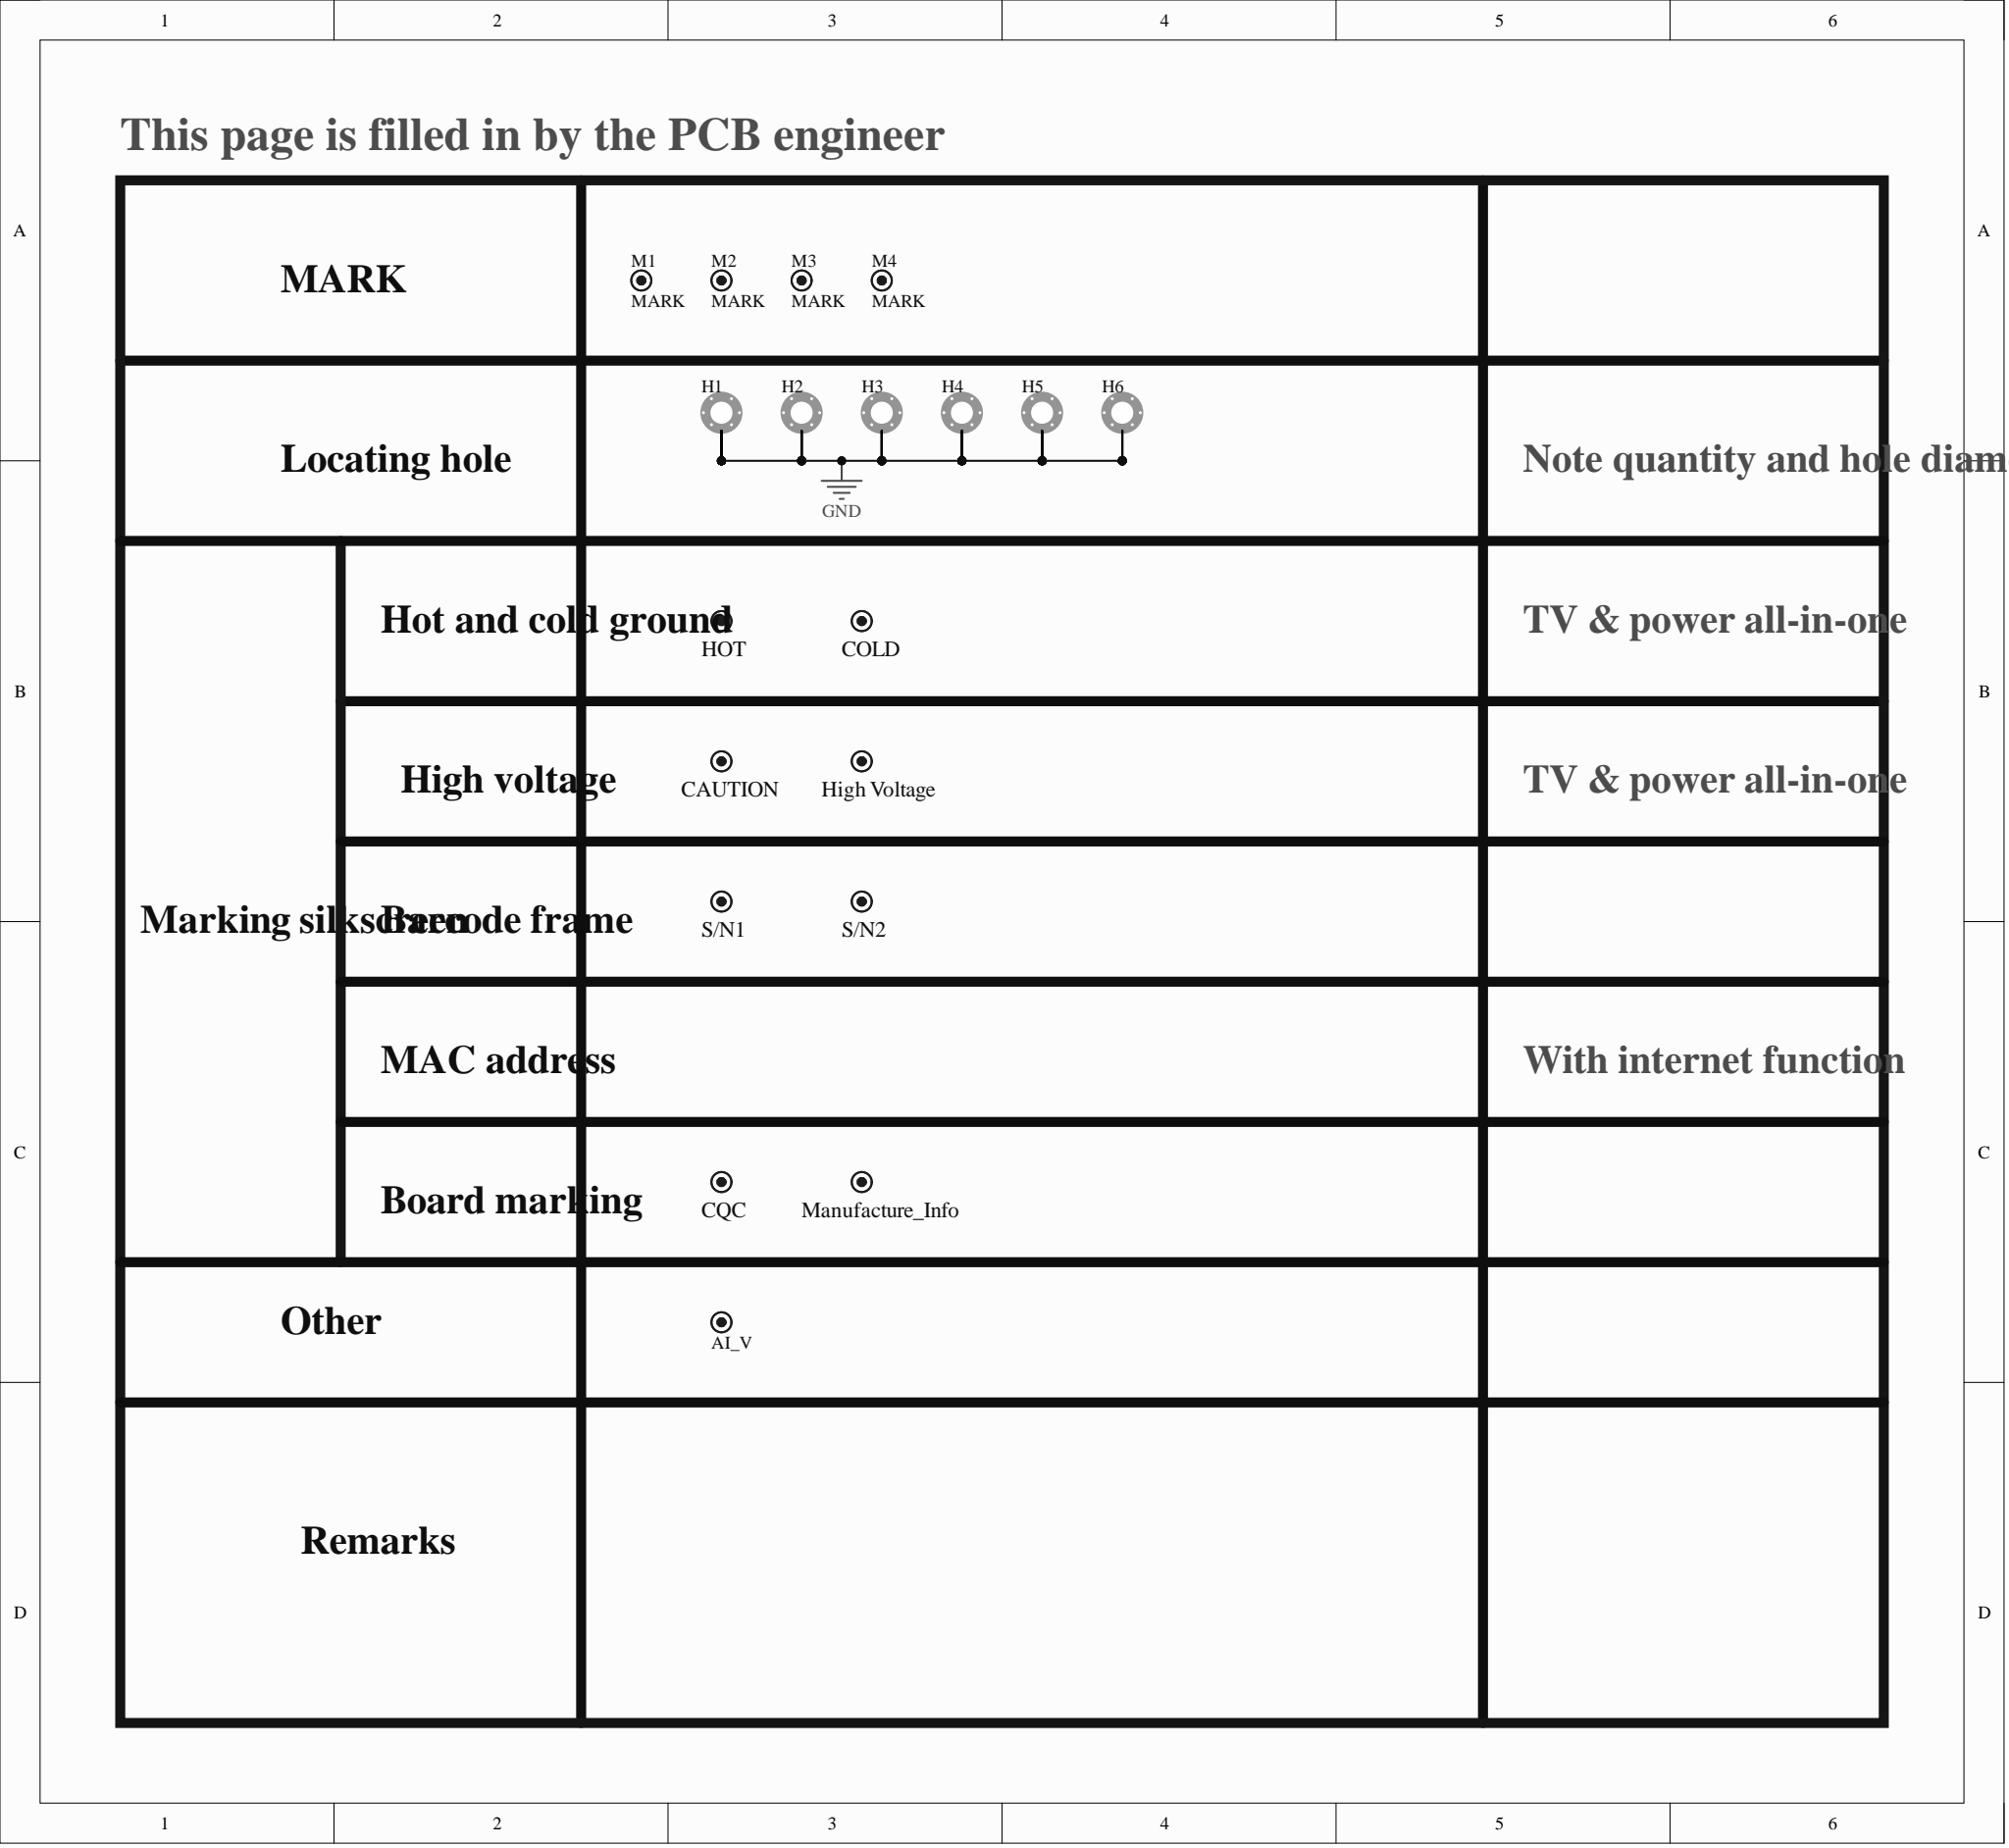Circuit board | Altium Designer | 574 parts | 274 nets | one sheet of the schematic
Parts on this sheet (reference | value | footprint):
AI_V | AI_GRIPPER_V | AI_GRIPPER_V
CAUTION | CAUTION | CAUTION
COLD | COLD | COLD
CQC | CQC | CQC
H1 | Location hole | ASSE4.0C-3
H2 | Location hole | ASSE4.0C-3
H3 | Location hole | ASSE4.0C-3
H4 | Location hole | ASSE4.0C-3
H5 | Location hole | ASSE4.0C-3
H6 | Location hole | ASSE4.0C-3
HOT | HOT | HOT
M1 | MARK | MARK
M2 | MARK | MARK
M3 | MARK | MARK
M4 | MARK | MARK
Manufacture_Info | Manufacture_Info | Manufacture_Info
S/N1 | Barcode | Barcode
S/N2 | Barcode | Barcode
Nets of these parts (net: part-pin ...):
GND: H1-1 H1-2 H1-3 H1-4 H1-5 H1-6 H2-1 H2-2 H2-3 H2-4 H2-5 H2-6 H3-1 H3-2 H3-3 H3-4 H3-5 H3-6 H4-1 H4-2 H4-3 H4-4 H4-5 H4-6 H5-1 H5-2 H5-3 H5-4 H5-5 H5-6 H6-1 H6-2 H6-3 H6-4 H6-5 H6-6